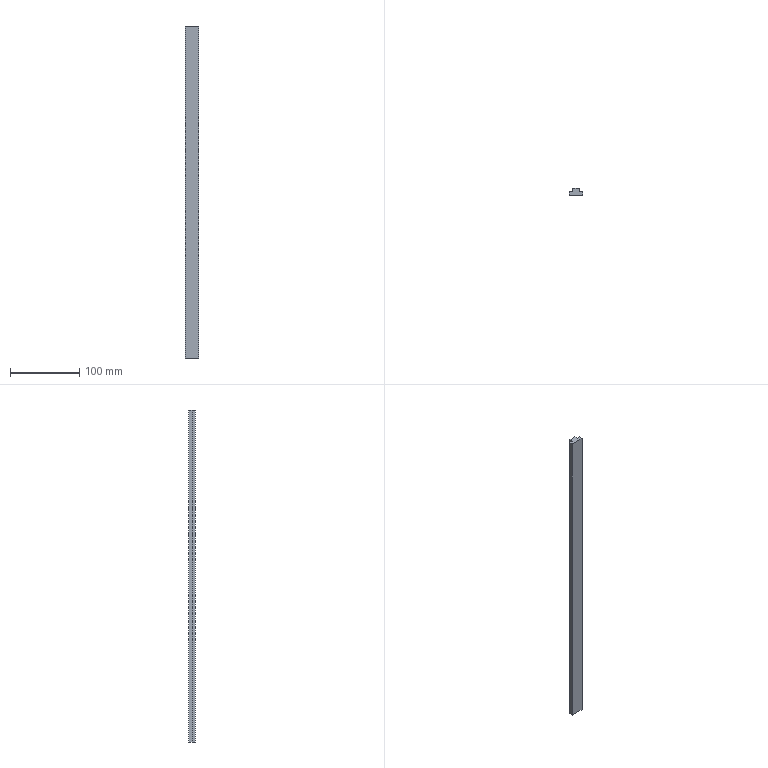Part | SolidWorks | features Extrusion 1 | 1 solid | 10 faces | box 20 x 10 x 480 mm | volume 72000 mm3 | plane 10
STEP:
#1=CARTESIAN_POINT('',(0.,5.,0.));
#2=VERTEX_POINT('',#1);
#3=CARTESIAN_POINT('',(0.,0.,0.));
#4=VERTEX_POINT('',#3);
#5=CARTESIAN_POINT('',(0.,0.,0.));
#6=DIRECTION('',(0.,-1.,0.));
#7=VECTOR('',#6,1000.);
#8=LINE('',#5,#7);
#9=EDGE_CURVE('',#2,#4,#8,.T.);
#10=ORIENTED_EDGE('',*,*,#9,.T.);
#11=CARTESIAN_POINT('',(0.,0.,480.));
#12=VERTEX_POINT('',#11);
#13=CARTESIAN_POINT('',(0.,0.,480.));
#14=DIRECTION('',(0.,0.,-1.));
#15=VECTOR('',#14,1000.);
#16=LINE('',#13,#15);
#17=EDGE_CURVE('',#12,#4,#16,.T.);
#18=ORIENTED_EDGE('',*,*,#17,.F.);
#19=CARTESIAN_POINT('',(0.,5.,480.));
#20=VERTEX_POINT('',#19);
#21=CARTESIAN_POINT('',(0.,0.,480.));
#22=DIRECTION('',(0.,-1.,0.));
#23=VECTOR('',#22,1000.);
#24=LINE('',#21,#23);
#25=EDGE_CURVE('',#20,#12,#24,.T.);
#26=ORIENTED_EDGE('',*,*,#25,.F.);
#27=CARTESIAN_POINT('',(0.,5.,480.));
#28=DIRECTION('',(0.,0.,-1.));
#29=VECTOR('',#28,1000.);
#30=LINE('',#27,#29);
#31=EDGE_CURVE('',#20,#2,#30,.T.);
#32=ORIENTED_EDGE('',*,*,#31,.T.);
#33=EDGE_LOOP('',(#10,#18,#26,#32));
#34=FACE_OUTER_BOUND('',#33,.T.);
#35=CARTESIAN_POINT('',(0.,0.,480.));
#36=DIRECTION('',(1.,0.,0.));
#37=DIRECTION('',(0.,0.,-1.));
#38=AXIS2_PLACEMENT_3D('',#35,#36,#37);
#39=PLANE('',#38);
#40=ADVANCED_FACE('',(#34),#39,.F.);
#41=CARTESIAN_POINT('',(20.,0.,0.));
#42=VERTEX_POINT('',#41);
#43=CARTESIAN_POINT('',(0.,0.,0.));
#44=DIRECTION('',(1.,0.,0.));
#45=VECTOR('',#44,1000.);
#46=LINE('',#43,#45);
#47=EDGE_CURVE('',#4,#42,#46,.T.);
#48=ORIENTED_EDGE('',*,*,#47,.T.);
#49=CARTESIAN_POINT('',(20.,0.,480.));
#50=VERTEX_POINT('',#49);
#51=CARTESIAN_POINT('',(20.,0.,480.));
#52=DIRECTION('',(0.,0.,-1.));
#53=VECTOR('',#52,1000.);
#54=LINE('',#51,#53);
#55=EDGE_CURVE('',#50,#42,#54,.T.);
#56=ORIENTED_EDGE('',*,*,#55,.F.);
#57=CARTESIAN_POINT('',(0.,0.,480.));
#58=DIRECTION('',(1.,0.,0.));
#59=VECTOR('',#58,1000.);
#60=LINE('',#57,#59);
#61=EDGE_CURVE('',#12,#50,#60,.T.);
#62=ORIENTED_EDGE('',*,*,#61,.F.);
#63=ORIENTED_EDGE('',*,*,#17,.T.);
#64=EDGE_LOOP('',(#48,#56,#62,#63));
#65=FACE_OUTER_BOUND('',#64,.T.);
#66=CARTESIAN_POINT('',(0.,0.,480.));
#67=DIRECTION('',(0.,1.,0.));
#68=DIRECTION('',(0.,0.,1.));
#69=AXIS2_PLACEMENT_3D('',#66,#67,#68);
#70=PLANE('',#69);
#71=ADVANCED_FACE('',(#65),#70,.F.);
#72=CARTESIAN_POINT('',(20.,5.,0.));
#73=VERTEX_POINT('',#72);
#74=CARTESIAN_POINT('',(20.,0.,0.));
#75=DIRECTION('',(0.,1.,0.));
#76=VECTOR('',#75,1000.);
#77=LINE('',#74,#76);
#78=EDGE_CURVE('',#42,#73,#77,.T.);
#79=ORIENTED_EDGE('',*,*,#78,.T.);
#80=CARTESIAN_POINT('',(20.,5.,480.));
#81=VERTEX_POINT('',#80);
#82=CARTESIAN_POINT('',(20.,5.,480.));
#83=DIRECTION('',(0.,0.,-1.));
#84=VECTOR('',#83,1000.);
#85=LINE('',#82,#84);
#86=EDGE_CURVE('',#81,#73,#85,.T.);
#87=ORIENTED_EDGE('',*,*,#86,.F.);
#88=CARTESIAN_POINT('',(20.,0.,480.));
#89=DIRECTION('',(0.,1.,0.));
#90=VECTOR('',#89,1000.);
#91=LINE('',#88,#90);
#92=EDGE_CURVE('',#50,#81,#91,.T.);
#93=ORIENTED_EDGE('',*,*,#92,.F.);
#94=ORIENTED_EDGE('',*,*,#55,.T.);
#95=EDGE_LOOP('',(#79,#87,#93,#94));
#96=FACE_OUTER_BOUND('',#95,.T.);
#97=CARTESIAN_POINT('',(20.,0.,480.));
#98=DIRECTION('',(-1.,0.,0.));
#99=DIRECTION('',(0.,0.,1.));
#100=AXIS2_PLACEMENT_3D('',#97,#98,#99);
#101=PLANE('',#100);
#102=ADVANCED_FACE('',(#96),#101,.F.);
#103=CARTESIAN_POINT('',(15.,5.,0.));
#104=VERTEX_POINT('',#103);
#105=CARTESIAN_POINT('',(15.,5.,0.));
#106=DIRECTION('',(-1.,0.,0.));
#107=VECTOR('',#106,1000.);
#108=LINE('',#105,#107);
#109=EDGE_CURVE('',#73,#104,#108,.T.);
#110=ORIENTED_EDGE('',*,*,#109,.T.);
#111=CARTESIAN_POINT('',(15.,5.,480.));
#112=VERTEX_POINT('',#111);
#113=CARTESIAN_POINT('',(15.,5.,480.));
#114=DIRECTION('',(0.,0.,-1.));
#115=VECTOR('',#114,1000.);
#116=LINE('',#113,#115);
#117=EDGE_CURVE('',#112,#104,#116,.T.);
#118=ORIENTED_EDGE('',*,*,#117,.F.);
#119=CARTESIAN_POINT('',(15.,5.,480.));
#120=DIRECTION('',(-1.,0.,0.));
#121=VECTOR('',#120,1000.);
#122=LINE('',#119,#121);
#123=EDGE_CURVE('',#81,#112,#122,.T.);
#124=ORIENTED_EDGE('',*,*,#123,.F.);
#125=ORIENTED_EDGE('',*,*,#86,.T.);
#126=EDGE_LOOP('',(#110,#118,#124,#125));
#127=FACE_OUTER_BOUND('',#126,.T.);
#128=CARTESIAN_POINT('',(15.,5.,480.));
#129=DIRECTION('',(0.,-1.,0.));
#130=DIRECTION('',(0.,0.,-1.));
#131=AXIS2_PLACEMENT_3D('',#128,#129,#130);
#132=PLANE('',#131);
#133=ADVANCED_FACE('',(#127),#132,.F.);
#134=CARTESIAN_POINT('',(15.,10.,0.));
#135=VERTEX_POINT('',#134);
#136=CARTESIAN_POINT('',(15.,10.,0.));
#137=DIRECTION('',(0.,1.,0.));
#138=VECTOR('',#137,1000.);
#139=LINE('',#136,#138);
#140=EDGE_CURVE('',#104,#135,#139,.T.);
#141=ORIENTED_EDGE('',*,*,#140,.T.);
#142=CARTESIAN_POINT('',(15.,10.,480.));
#143=VERTEX_POINT('',#142);
#144=CARTESIAN_POINT('',(15.,10.,480.));
#145=DIRECTION('',(0.,0.,-1.));
#146=VECTOR('',#145,1000.);
#147=LINE('',#144,#146);
#148=EDGE_CURVE('',#143,#135,#147,.T.);
#149=ORIENTED_EDGE('',*,*,#148,.F.);
#150=CARTESIAN_POINT('',(15.,10.,480.));
#151=DIRECTION('',(0.,1.,0.));
#152=VECTOR('',#151,1000.);
#153=LINE('',#150,#152);
#154=EDGE_CURVE('',#112,#143,#153,.T.);
#155=ORIENTED_EDGE('',*,*,#154,.F.);
#156=ORIENTED_EDGE('',*,*,#117,.T.);
#157=EDGE_LOOP('',(#141,#149,#155,#156));
#158=FACE_OUTER_BOUND('',#157,.T.);
#159=CARTESIAN_POINT('',(15.,10.,480.));
#160=DIRECTION('',(-1.,0.,0.));
#161=DIRECTION('',(0.,0.,1.));
#162=AXIS2_PLACEMENT_3D('',#159,#160,#161);
#163=PLANE('',#162);
#164=ADVANCED_FACE('',(#158),#163,.F.);
#165=CARTESIAN_POINT('',(5.,10.,0.));
#166=VERTEX_POINT('',#165);
#167=CARTESIAN_POINT('',(5.,10.,0.));
#168=DIRECTION('',(-1.,0.,0.));
#169=VECTOR('',#168,1000.);
#170=LINE('',#167,#169);
#171=EDGE_CURVE('',#135,#166,#170,.T.);
#172=ORIENTED_EDGE('',*,*,#171,.T.);
#173=CARTESIAN_POINT('',(5.,10.,480.));
#174=VERTEX_POINT('',#173);
#175=CARTESIAN_POINT('',(5.,10.,480.));
#176=DIRECTION('',(0.,0.,-1.));
#177=VECTOR('',#176,1000.);
#178=LINE('',#175,#177);
#179=EDGE_CURVE('',#174,#166,#178,.T.);
#180=ORIENTED_EDGE('',*,*,#179,.F.);
#181=CARTESIAN_POINT('',(5.,10.,480.));
#182=DIRECTION('',(-1.,0.,0.));
#183=VECTOR('',#182,1000.);
#184=LINE('',#181,#183);
#185=EDGE_CURVE('',#143,#174,#184,.T.);
#186=ORIENTED_EDGE('',*,*,#185,.F.);
#187=ORIENTED_EDGE('',*,*,#148,.T.);
#188=EDGE_LOOP('',(#172,#180,#186,#187));
#189=FACE_OUTER_BOUND('',#188,.T.);
#190=CARTESIAN_POINT('',(5.,10.,480.));
#191=DIRECTION('',(0.,-1.,0.));
#192=DIRECTION('',(0.,0.,-1.));
#193=AXIS2_PLACEMENT_3D('',#190,#191,#192);
#194=PLANE('',#193);
#195=ADVANCED_FACE('',(#189),#194,.F.);
#196=CARTESIAN_POINT('',(5.,5.,0.));
#197=VERTEX_POINT('',#196);
#198=CARTESIAN_POINT('',(5.,5.,0.));
#199=DIRECTION('',(0.,-1.,0.));
#200=VECTOR('',#199,1000.);
#201=LINE('',#198,#200);
#202=EDGE_CURVE('',#166,#197,#201,.T.);
#203=ORIENTED_EDGE('',*,*,#202,.T.);
#204=CARTESIAN_POINT('',(5.,5.,480.));
#205=VERTEX_POINT('',#204);
#206=CARTESIAN_POINT('',(5.,5.,480.));
#207=DIRECTION('',(0.,0.,-1.));
#208=VECTOR('',#207,1000.);
#209=LINE('',#206,#208);
#210=EDGE_CURVE('',#205,#197,#209,.T.);
#211=ORIENTED_EDGE('',*,*,#210,.F.);
#212=CARTESIAN_POINT('',(5.,5.,480.));
#213=DIRECTION('',(0.,-1.,0.));
#214=VECTOR('',#213,1000.);
#215=LINE('',#212,#214);
#216=EDGE_CURVE('',#174,#205,#215,.T.);
#217=ORIENTED_EDGE('',*,*,#216,.F.);
#218=ORIENTED_EDGE('',*,*,#179,.T.);
#219=EDGE_LOOP('',(#203,#211,#217,#218));
#220=FACE_OUTER_BOUND('',#219,.T.);
#221=CARTESIAN_POINT('',(5.,5.,480.));
#222=DIRECTION('',(1.,0.,0.));
#223=DIRECTION('',(0.,1.,0.));
#224=AXIS2_PLACEMENT_3D('',#221,#222,#223);
#225=PLANE('',#224);
#226=ADVANCED_FACE('',(#220),#225,.F.);
#227=CARTESIAN_POINT('',(0.,5.,0.));
#228=DIRECTION('',(-1.,0.,0.));
#229=VECTOR('',#228,1000.);
#230=LINE('',#227,#229);
#231=EDGE_CURVE('',#197,#2,#230,.T.);
#232=ORIENTED_EDGE('',*,*,#231,.T.);
#233=ORIENTED_EDGE('',*,*,#31,.F.);
#234=CARTESIAN_POINT('',(0.,5.,480.));
#235=DIRECTION('',(-1.,0.,0.));
#236=VECTOR('',#235,1000.);
#237=LINE('',#234,#236);
#238=EDGE_CURVE('',#205,#20,#237,.T.);
#239=ORIENTED_EDGE('',*,*,#238,.F.);
#240=ORIENTED_EDGE('',*,*,#210,.T.);
#241=EDGE_LOOP('',(#232,#233,#239,#240));
#242=FACE_OUTER_BOUND('',#241,.T.);
#243=CARTESIAN_POINT('',(0.,5.,480.));
#244=DIRECTION('',(0.,-1.,0.));
#245=DIRECTION('',(0.,0.,-1.));
#246=AXIS2_PLACEMENT_3D('',#243,#244,#245);
#247=PLANE('',#246);
#248=ADVANCED_FACE('',(#242),#247,.F.);
#249=ORIENTED_EDGE('',*,*,#25,.T.);
#250=ORIENTED_EDGE('',*,*,#61,.T.);
#251=ORIENTED_EDGE('',*,*,#92,.T.);
#252=ORIENTED_EDGE('',*,*,#123,.T.);
#253=ORIENTED_EDGE('',*,*,#154,.T.);
#254=ORIENTED_EDGE('',*,*,#185,.T.);
#255=ORIENTED_EDGE('',*,*,#216,.T.);
#256=ORIENTED_EDGE('',*,*,#238,.T.);
#257=EDGE_LOOP('',(#249,#250,#251,#252,#253,#254,#255,#256));
#258=FACE_OUTER_BOUND('',#257,.T.);
#259=CARTESIAN_POINT('',(0.,0.,480.));
#260=DIRECTION('',(0.,0.,-1.));
#261=DIRECTION('',(-1.,0.,0.));
#262=AXIS2_PLACEMENT_3D('',#259,#260,#261);
#263=PLANE('',#262);
#264=ADVANCED_FACE('',(#258),#263,.F.);
#265=ORIENTED_EDGE('',*,*,#9,.F.);
#266=ORIENTED_EDGE('',*,*,#231,.F.);
#267=ORIENTED_EDGE('',*,*,#202,.F.);
#268=ORIENTED_EDGE('',*,*,#171,.F.);
#269=ORIENTED_EDGE('',*,*,#140,.F.);
#270=ORIENTED_EDGE('',*,*,#109,.F.);
#271=ORIENTED_EDGE('',*,*,#78,.F.);
#272=ORIENTED_EDGE('',*,*,#47,.F.);
#273=EDGE_LOOP('',(#265,#266,#267,#268,#269,#270,#271,#272));
#274=FACE_OUTER_BOUND('',#273,.T.);
#275=CARTESIAN_POINT('',(0.,0.,0.));
#276=DIRECTION('',(0.,0.,-1.));
#277=DIRECTION('',(-1.,0.,0.));
#278=AXIS2_PLACEMENT_3D('',#275,#276,#277);
#279=PLANE('',#278);
#280=ADVANCED_FACE('',(#274),#279,.T.);
#281=CLOSED_SHELL('',(#40,#71,#102,#133,#164,#195,#226,#248,#264,#280));
#282=MANIFOLD_SOLID_BREP('',#281);
#283=CARTESIAN_POINT('',(0.,0.,0.));
#284=DIRECTION('',(0.,0.,1.));
#285=DIRECTION('',(1.,0.,0.));
#286=AXIS2_PLACEMENT_3D('',#283,#284,#285);
#287=(LENGTH_UNIT()NAMED_UNIT(*)SI_UNIT(.MILLI.,.METRE.));
#288=UNCERTAINTY_MEASURE_WITH_UNIT(LENGTH_MEASURE(0.00001),#287,'','');
#289=(NAMED_UNIT(*)PLANE_ANGLE_UNIT()SI_UNIT($,.RADIAN.));
#290=(NAMED_UNIT(*)SI_UNIT($,.STERADIAN.)SOLID_ANGLE_UNIT());
#291=(GEOMETRIC_REPRESENTATION_CONTEXT(3)GLOBAL_UNCERTAINTY_ASSIGNED_CONTEXT((#288))GLOBAL_UNIT_ASSIGNED_CONTEXT((#287,#289,#290))REPRESENTATION_CONTEXT('',''));
#292=ADVANCED_BREP_SHAPE_REPRESENTATION('',(#282,#286),#291);